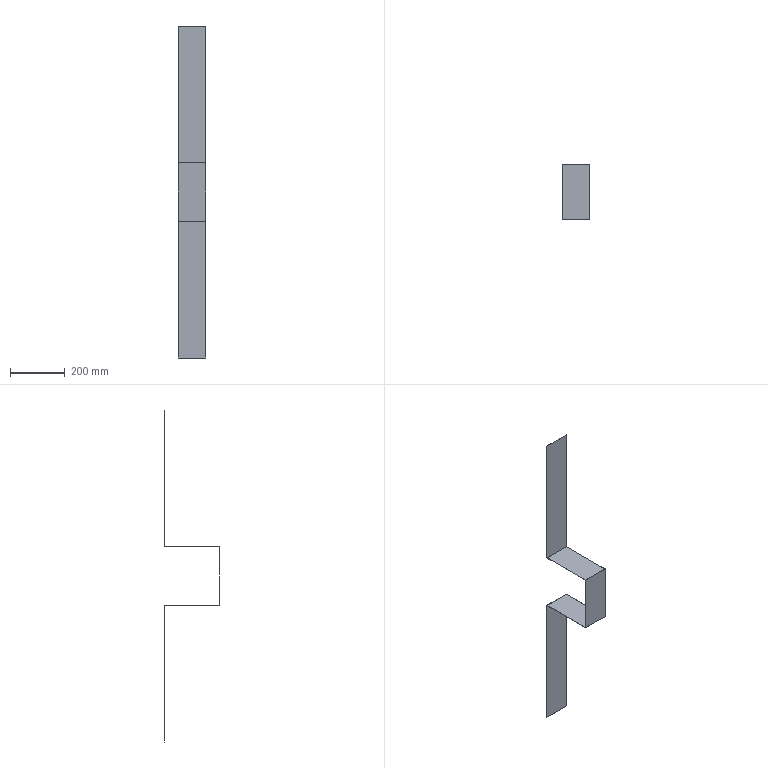Part | STEP file | 1 solid | 14 faces | box 100 x 200.5 x 1212 mm | volume 80600 mm3 | plane 14
STEP:
#1=CARTESIAN_POINT('',(0.,0.,0.));
#2=DIRECTION('',(0.,0.,1.));
#3=DIRECTION('',(1.,0.,0.));
#4=AXIS2_PLACEMENT_3D('',#1,#2,#3);
#5=CARTESIAN_POINT('',(-50.,0.25,0.));
#6=VERTEX_POINT('',#5);
#7=CARTESIAN_POINT('',(-50.,-0.25,0.));
#8=VERTEX_POINT('',#7);
#9=CARTESIAN_POINT('',(-50.,0.25,0.));
#10=DIRECTION('',(0.,-1.,0.));
#11=VECTOR('',#10,1.);
#12=LINE('',#9,#11);
#13=CARTESIAN_POINT('',(50.,0.25,0.));
#14=DIRECTION('',(0.,0.,-1.));
#15=DIRECTION('',(-1.,0.,0.));
#16=AXIS2_PLACEMENT_3D('',#13,#14,#15);
#17=PLANE('',#16);
#18=CARTESIAN_POINT('',(100.,0.));
#19=DIRECTION('',(0.,-1.));
#20=VECTOR('',#19,1.);
#21=LINE('',#18,#20);
#22=(GEOMETRIC_REPRESENTATION_CONTEXT(2)PARAMETRIC_REPRESENTATION_CONTEXT()REPRESENTATION_CONTEXT('',''));
#23=DEFINITIONAL_REPRESENTATION('',(#21),#22);
#24=PCURVE('',#17,#23);
#25=CARTESIAN_POINT('',(-50.,0.,0.));
#26=DIRECTION('',(1.,0.,0.));
#27=DIRECTION('',(0.,0.,-1.));
#28=AXIS2_PLACEMENT_3D('',#25,#26,#27);
#29=PLANE('',#28);
#30=CARTESIAN_POINT('',(0.,0.25));
#31=DIRECTION('',(0.,-1.));
#32=VECTOR('',#31,1.);
#33=LINE('',#30,#32);
#34=(GEOMETRIC_REPRESENTATION_CONTEXT(2)PARAMETRIC_REPRESENTATION_CONTEXT()REPRESENTATION_CONTEXT('',''));
#35=DEFINITIONAL_REPRESENTATION('',(#33),#34);
#36=PCURVE('',#29,#35);
#37=SURFACE_CURVE('',#12,(#24,#36),.PCURVE_S1.);
#38=EDGE_CURVE('',#6,#8,#37,.T.);
#39=ORIENTED_EDGE('',*,*,#38,.T.);
#40=CARTESIAN_POINT('',(50.,-0.25,0.));
#41=VERTEX_POINT('',#40);
#42=CARTESIAN_POINT('',(50.,-0.25,0.));
#43=DIRECTION('',(-1.,0.,0.));
#44=VECTOR('',#43,1.);
#45=LINE('',#42,#44);
#46=CARTESIAN_POINT('',(0.,-0.5));
#47=DIRECTION('',(1.,0.));
#48=VECTOR('',#47,1.);
#49=LINE('',#46,#48);
#50=(GEOMETRIC_REPRESENTATION_CONTEXT(2)PARAMETRIC_REPRESENTATION_CONTEXT()REPRESENTATION_CONTEXT('',''));
#51=DEFINITIONAL_REPRESENTATION('',(#49),#50);
#52=PCURVE('',#17,#51);
#53=CARTESIAN_POINT('',(50.,-0.25,0.));
#54=DIRECTION('',(0.,1.,0.));
#55=DIRECTION('',(0.,0.,1.));
#56=AXIS2_PLACEMENT_3D('',#53,#54,#55);
#57=PLANE('',#56);
#58=CARTESIAN_POINT('',(0.,0.));
#59=DIRECTION('',(0.,-1.));
#60=VECTOR('',#59,1.);
#61=LINE('',#58,#60);
#62=(GEOMETRIC_REPRESENTATION_CONTEXT(2)PARAMETRIC_REPRESENTATION_CONTEXT()REPRESENTATION_CONTEXT('',''));
#63=DEFINITIONAL_REPRESENTATION('',(#61),#62);
#64=PCURVE('',#57,#63);
#65=SURFACE_CURVE('',#45,(#52,#64),.PCURVE_S1.);
#66=EDGE_CURVE('',#41,#8,#65,.T.);
#67=ORIENTED_EDGE('',*,*,#66,.F.);
#68=CARTESIAN_POINT('',(50.,0.25,0.));
#69=VERTEX_POINT('',#68);
#70=CARTESIAN_POINT('',(50.,0.25,0.));
#71=DIRECTION('',(0.,-1.,0.));
#72=VECTOR('',#71,1.);
#73=LINE('',#70,#72);
#74=CARTESIAN_POINT('',(0.,0.));
#75=DIRECTION('',(0.,-1.));
#76=VECTOR('',#75,1.);
#77=LINE('',#74,#76);
#78=(GEOMETRIC_REPRESENTATION_CONTEXT(2)PARAMETRIC_REPRESENTATION_CONTEXT()REPRESENTATION_CONTEXT('',''));
#79=DEFINITIONAL_REPRESENTATION('',(#77),#78);
#80=PCURVE('',#17,#79);
#81=CARTESIAN_POINT('',(50.,0.,0.));
#82=DIRECTION('',(1.,0.,0.));
#83=DIRECTION('',(0.,0.,-1.));
#84=AXIS2_PLACEMENT_3D('',#81,#82,#83);
#85=PLANE('',#84);
#86=CARTESIAN_POINT('',(0.,0.25));
#87=DIRECTION('',(0.,-1.));
#88=VECTOR('',#87,1.);
#89=LINE('',#86,#88);
#90=(GEOMETRIC_REPRESENTATION_CONTEXT(2)PARAMETRIC_REPRESENTATION_CONTEXT()REPRESENTATION_CONTEXT('',''));
#91=DEFINITIONAL_REPRESENTATION('',(#89),#90);
#92=PCURVE('',#85,#91);
#93=SURFACE_CURVE('',#73,(#80,#92),.PCURVE_S1.);
#94=EDGE_CURVE('',#69,#41,#93,.T.);
#95=ORIENTED_EDGE('',*,*,#94,.F.);
#96=CARTESIAN_POINT('',(50.,0.25,0.));
#97=DIRECTION('',(-1.,0.,0.));
#98=VECTOR('',#97,1.);
#99=LINE('',#96,#98);
#100=CARTESIAN_POINT('',(0.,0.));
#101=DIRECTION('',(1.,0.));
#102=VECTOR('',#101,1.);
#103=LINE('',#100,#102);
#104=(GEOMETRIC_REPRESENTATION_CONTEXT(2)PARAMETRIC_REPRESENTATION_CONTEXT()REPRESENTATION_CONTEXT('',''));
#105=DEFINITIONAL_REPRESENTATION('',(#103),#104);
#106=PCURVE('',#17,#105);
#107=CARTESIAN_POINT('',(50.,0.25,0.));
#108=DIRECTION('',(0.,-1.,0.));
#109=DIRECTION('',(0.,0.,-1.));
#110=AXIS2_PLACEMENT_3D('',#107,#108,#109);
#111=PLANE('',#110);
#112=CARTESIAN_POINT('',(0.,0.));
#113=DIRECTION('',(0.,-1.));
#114=VECTOR('',#113,1.);
#115=LINE('',#112,#114);
#116=(GEOMETRIC_REPRESENTATION_CONTEXT(2)PARAMETRIC_REPRESENTATION_CONTEXT()REPRESENTATION_CONTEXT('',''));
#117=DEFINITIONAL_REPRESENTATION('',(#115),#116);
#118=PCURVE('',#111,#117);
#119=SURFACE_CURVE('',#99,(#106,#118),.PCURVE_S1.);
#120=EDGE_CURVE('',#69,#6,#119,.T.);
#121=ORIENTED_EDGE('',*,*,#120,.T.);
#122=EDGE_LOOP('',(#39,#67,#95,#121));
#123=FACE_BOUND('',#122,.T.);
#124=ADVANCED_FACE('',(#123),#17,.F.);
#125=CARTESIAN_POINT('',(-50.,-0.25,-499.5));
#126=VERTEX_POINT('',#125);
#127=CARTESIAN_POINT('',(-50.,-0.25,0.));
#128=DIRECTION('',(0.,0.,-1.));
#129=VECTOR('',#128,1.);
#130=LINE('',#127,#129);
#131=CARTESIAN_POINT('',(0.,-100.));
#132=DIRECTION('',(-1.,0.));
#133=VECTOR('',#132,1.);
#134=LINE('',#131,#133);
#135=(GEOMETRIC_REPRESENTATION_CONTEXT(2)PARAMETRIC_REPRESENTATION_CONTEXT()REPRESENTATION_CONTEXT('',''));
#136=DEFINITIONAL_REPRESENTATION('',(#134),#135);
#137=PCURVE('',#57,#136);
#138=CARTESIAN_POINT('',(0.,-0.25));
#139=DIRECTION('',(1.,0.));
#140=VECTOR('',#139,1.);
#141=LINE('',#138,#140);
#142=(GEOMETRIC_REPRESENTATION_CONTEXT(2)PARAMETRIC_REPRESENTATION_CONTEXT()REPRESENTATION_CONTEXT('',''));
#143=DEFINITIONAL_REPRESENTATION('',(#141),#142);
#144=PCURVE('',#29,#143);
#145=SURFACE_CURVE('',#130,(#137,#144),.PCURVE_S1.);
#146=EDGE_CURVE('',#8,#126,#145,.T.);
#147=ORIENTED_EDGE('',*,*,#146,.T.);
#148=CARTESIAN_POINT('',(50.,-0.25,-499.5));
#149=VERTEX_POINT('',#148);
#150=CARTESIAN_POINT('',(50.,-0.25,-499.5));
#151=DIRECTION('',(-1.,0.,0.));
#152=VECTOR('',#151,1.);
#153=LINE('',#150,#152);
#154=CARTESIAN_POINT('',(-499.5,0.));
#155=DIRECTION('',(0.,-1.));
#156=VECTOR('',#155,1.);
#157=LINE('',#154,#156);
#158=(GEOMETRIC_REPRESENTATION_CONTEXT(2)PARAMETRIC_REPRESENTATION_CONTEXT()REPRESENTATION_CONTEXT('',''));
#159=DEFINITIONAL_REPRESENTATION('',(#157),#158);
#160=PCURVE('',#57,#159);
#161=CARTESIAN_POINT('',(50.,-0.25,-499.5));
#162=DIRECTION('',(0.,0.,-1.));
#163=DIRECTION('',(-1.,0.,0.));
#164=AXIS2_PLACEMENT_3D('',#161,#162,#163);
#165=PLANE('',#164);
#166=CARTESIAN_POINT('',(0.,0.));
#167=DIRECTION('',(1.,0.));
#168=VECTOR('',#167,1.);
#169=LINE('',#166,#168);
#170=(GEOMETRIC_REPRESENTATION_CONTEXT(2)PARAMETRIC_REPRESENTATION_CONTEXT()REPRESENTATION_CONTEXT('',''));
#171=DEFINITIONAL_REPRESENTATION('',(#169),#170);
#172=PCURVE('',#165,#171);
#173=SURFACE_CURVE('',#153,(#160,#172),.PCURVE_S1.);
#174=EDGE_CURVE('',#149,#126,#173,.T.);
#175=ORIENTED_EDGE('',*,*,#174,.F.);
#176=CARTESIAN_POINT('',(50.,-0.25,0.));
#177=DIRECTION('',(0.,0.,-1.));
#178=VECTOR('',#177,1.);
#179=LINE('',#176,#178);
#180=CARTESIAN_POINT('',(0.,0.));
#181=DIRECTION('',(-1.,0.));
#182=VECTOR('',#181,1.);
#183=LINE('',#180,#182);
#184=(GEOMETRIC_REPRESENTATION_CONTEXT(2)PARAMETRIC_REPRESENTATION_CONTEXT()REPRESENTATION_CONTEXT('',''));
#185=DEFINITIONAL_REPRESENTATION('',(#183),#184);
#186=PCURVE('',#57,#185);
#187=CARTESIAN_POINT('',(0.,-0.25));
#188=DIRECTION('',(1.,0.));
#189=VECTOR('',#188,1.);
#190=LINE('',#187,#189);
#191=(GEOMETRIC_REPRESENTATION_CONTEXT(2)PARAMETRIC_REPRESENTATION_CONTEXT()REPRESENTATION_CONTEXT('',''));
#192=DEFINITIONAL_REPRESENTATION('',(#190),#191);
#193=PCURVE('',#85,#192);
#194=SURFACE_CURVE('',#179,(#186,#193),.PCURVE_S1.);
#195=EDGE_CURVE('',#41,#149,#194,.T.);
#196=ORIENTED_EDGE('',*,*,#195,.F.);
#197=ORIENTED_EDGE('',*,*,#66,.T.);
#198=EDGE_LOOP('',(#147,#175,#196,#197));
#199=FACE_BOUND('',#198,.T.);
#200=ADVANCED_FACE('',(#199),#57,.F.);
#201=CARTESIAN_POINT('',(-50.,-200.25,-499.5));
#202=VERTEX_POINT('',#201);
#203=CARTESIAN_POINT('',(-50.,-0.25,-499.5));
#204=DIRECTION('',(0.,-1.,0.));
#205=VECTOR('',#204,1.);
#206=LINE('',#203,#205);
#207=CARTESIAN_POINT('',(100.,0.));
#208=DIRECTION('',(0.,-1.));
#209=VECTOR('',#208,1.);
#210=LINE('',#207,#209);
#211=(GEOMETRIC_REPRESENTATION_CONTEXT(2)PARAMETRIC_REPRESENTATION_CONTEXT()REPRESENTATION_CONTEXT('',''));
#212=DEFINITIONAL_REPRESENTATION('',(#210),#211);
#213=PCURVE('',#165,#212);
#214=CARTESIAN_POINT('',(499.5,-0.25));
#215=DIRECTION('',(0.,-1.));
#216=VECTOR('',#215,1.);
#217=LINE('',#214,#216);
#218=(GEOMETRIC_REPRESENTATION_CONTEXT(2)PARAMETRIC_REPRESENTATION_CONTEXT()REPRESENTATION_CONTEXT('',''));
#219=DEFINITIONAL_REPRESENTATION('',(#217),#218);
#220=PCURVE('',#29,#219);
#221=SURFACE_CURVE('',#206,(#213,#220),.PCURVE_S1.);
#222=EDGE_CURVE('',#126,#202,#221,.T.);
#223=ORIENTED_EDGE('',*,*,#222,.T.);
#224=CARTESIAN_POINT('',(50.,-200.25,-499.5));
#225=VERTEX_POINT('',#224);
#226=CARTESIAN_POINT('',(50.,-200.25,-499.5));
#227=DIRECTION('',(-1.,0.,0.));
#228=VECTOR('',#227,1.);
#229=LINE('',#226,#228);
#230=CARTESIAN_POINT('',(0.,-200.));
#231=DIRECTION('',(1.,0.));
#232=VECTOR('',#231,1.);
#233=LINE('',#230,#232);
#234=(GEOMETRIC_REPRESENTATION_CONTEXT(2)PARAMETRIC_REPRESENTATION_CONTEXT()REPRESENTATION_CONTEXT('',''));
#235=DEFINITIONAL_REPRESENTATION('',(#233),#234);
#236=PCURVE('',#165,#235);
#237=CARTESIAN_POINT('',(50.,-200.25,-499.5));
#238=DIRECTION('',(0.,1.,0.));
#239=DIRECTION('',(0.,0.,1.));
#240=AXIS2_PLACEMENT_3D('',#237,#238,#239);
#241=PLANE('',#240);
#242=CARTESIAN_POINT('',(0.,0.));
#243=DIRECTION('',(0.,-1.));
#244=VECTOR('',#243,1.);
#245=LINE('',#242,#244);
#246=(GEOMETRIC_REPRESENTATION_CONTEXT(2)PARAMETRIC_REPRESENTATION_CONTEXT()REPRESENTATION_CONTEXT('',''));
#247=DEFINITIONAL_REPRESENTATION('',(#245),#246);
#248=PCURVE('',#241,#247);
#249=SURFACE_CURVE('',#229,(#236,#248),.PCURVE_S1.);
#250=EDGE_CURVE('',#225,#202,#249,.T.);
#251=ORIENTED_EDGE('',*,*,#250,.F.);
#252=CARTESIAN_POINT('',(50.,-0.25,-499.5));
#253=DIRECTION('',(0.,-1.,0.));
#254=VECTOR('',#253,1.);
#255=LINE('',#252,#254);
#256=CARTESIAN_POINT('',(0.,0.));
#257=DIRECTION('',(0.,-1.));
#258=VECTOR('',#257,1.);
#259=LINE('',#256,#258);
#260=(GEOMETRIC_REPRESENTATION_CONTEXT(2)PARAMETRIC_REPRESENTATION_CONTEXT()REPRESENTATION_CONTEXT('',''));
#261=DEFINITIONAL_REPRESENTATION('',(#259),#260);
#262=PCURVE('',#165,#261);
#263=CARTESIAN_POINT('',(499.5,-0.25));
#264=DIRECTION('',(0.,-1.));
#265=VECTOR('',#264,1.);
#266=LINE('',#263,#265);
#267=(GEOMETRIC_REPRESENTATION_CONTEXT(2)PARAMETRIC_REPRESENTATION_CONTEXT()REPRESENTATION_CONTEXT('',''));
#268=DEFINITIONAL_REPRESENTATION('',(#266),#267);
#269=PCURVE('',#85,#268);
#270=SURFACE_CURVE('',#255,(#262,#269),.PCURVE_S1.);
#271=EDGE_CURVE('',#149,#225,#270,.T.);
#272=ORIENTED_EDGE('',*,*,#271,.F.);
#273=ORIENTED_EDGE('',*,*,#174,.T.);
#274=EDGE_LOOP('',(#223,#251,#272,#273));
#275=FACE_BOUND('',#274,.T.);
#276=ADVANCED_FACE('',(#275),#165,.F.);
#277=CARTESIAN_POINT('',(-50.,-200.25,-712.5));
#278=VERTEX_POINT('',#277);
#279=CARTESIAN_POINT('',(-50.,-200.25,-499.5));
#280=DIRECTION('',(0.,0.,-1.));
#281=VECTOR('',#280,1.);
#282=LINE('',#279,#281);
#283=CARTESIAN_POINT('',(0.,-100.));
#284=DIRECTION('',(-1.,0.));
#285=VECTOR('',#284,1.);
#286=LINE('',#283,#285);
#287=(GEOMETRIC_REPRESENTATION_CONTEXT(2)PARAMETRIC_REPRESENTATION_CONTEXT()REPRESENTATION_CONTEXT('',''));
#288=DEFINITIONAL_REPRESENTATION('',(#286),#287);
#289=PCURVE('',#241,#288);
#290=CARTESIAN_POINT('',(499.5,-200.25));
#291=DIRECTION('',(1.,0.));
#292=VECTOR('',#291,1.);
#293=LINE('',#290,#292);
#294=(GEOMETRIC_REPRESENTATION_CONTEXT(2)PARAMETRIC_REPRESENTATION_CONTEXT()REPRESENTATION_CONTEXT('',''));
#295=DEFINITIONAL_REPRESENTATION('',(#293),#294);
#296=PCURVE('',#29,#295);
#297=SURFACE_CURVE('',#282,(#289,#296),.PCURVE_S1.);
#298=EDGE_CURVE('',#202,#278,#297,.T.);
#299=ORIENTED_EDGE('',*,*,#298,.T.);
#300=CARTESIAN_POINT('',(50.,-200.25,-712.5));
#301=VERTEX_POINT('',#300);
#302=CARTESIAN_POINT('',(50.,-200.25,-712.5));
#303=DIRECTION('',(-1.,0.,0.));
#304=VECTOR('',#303,1.);
#305=LINE('',#302,#304);
#306=CARTESIAN_POINT('',(-213.,0.));
#307=DIRECTION('',(0.,-1.));
#308=VECTOR('',#307,1.);
#309=LINE('',#306,#308);
#310=(GEOMETRIC_REPRESENTATION_CONTEXT(2)PARAMETRIC_REPRESENTATION_CONTEXT()REPRESENTATION_CONTEXT('',''));
#311=DEFINITIONAL_REPRESENTATION('',(#309),#310);
#312=PCURVE('',#241,#311);
#313=CARTESIAN_POINT('',(50.,-200.25,-712.5));
#314=DIRECTION('',(0.,0.,1.));
#315=DIRECTION('',(1.,0.,0.));
#316=AXIS2_PLACEMENT_3D('',#313,#314,#315);
#317=PLANE('',#316);
#318=CARTESIAN_POINT('',(0.,0.));
#319=DIRECTION('',(-1.,0.));
#320=VECTOR('',#319,1.);
#321=LINE('',#318,#320);
#322=(GEOMETRIC_REPRESENTATION_CONTEXT(2)PARAMETRIC_REPRESENTATION_CONTEXT()REPRESENTATION_CONTEXT('',''));
#323=DEFINITIONAL_REPRESENTATION('',(#321),#322);
#324=PCURVE('',#317,#323);
#325=SURFACE_CURVE('',#305,(#312,#324),.PCURVE_S1.);
#326=EDGE_CURVE('',#301,#278,#325,.T.);
#327=ORIENTED_EDGE('',*,*,#326,.F.);
#328=CARTESIAN_POINT('',(50.,-200.25,-499.5));
#329=DIRECTION('',(0.,0.,-1.));
#330=VECTOR('',#329,1.);
#331=LINE('',#328,#330);
#332=CARTESIAN_POINT('',(0.,0.));
#333=DIRECTION('',(-1.,0.));
#334=VECTOR('',#333,1.);
#335=LINE('',#332,#334);
#336=(GEOMETRIC_REPRESENTATION_CONTEXT(2)PARAMETRIC_REPRESENTATION_CONTEXT()REPRESENTATION_CONTEXT('',''));
#337=DEFINITIONAL_REPRESENTATION('',(#335),#336);
#338=PCURVE('',#241,#337);
#339=CARTESIAN_POINT('',(499.5,-200.25));
#340=DIRECTION('',(1.,0.));
#341=VECTOR('',#340,1.);
#342=LINE('',#339,#341);
#343=(GEOMETRIC_REPRESENTATION_CONTEXT(2)PARAMETRIC_REPRESENTATION_CONTEXT()REPRESENTATION_CONTEXT('',''));
#344=DEFINITIONAL_REPRESENTATION('',(#342),#343);
#345=PCURVE('',#85,#344);
#346=SURFACE_CURVE('',#331,(#338,#345),.PCURVE_S1.);
#347=EDGE_CURVE('',#225,#301,#346,.T.);
#348=ORIENTED_EDGE('',*,*,#347,.F.);
#349=ORIENTED_EDGE('',*,*,#250,.T.);
#350=EDGE_LOOP('',(#299,#327,#348,#349));
#351=FACE_BOUND('',#350,.T.);
#352=ADVANCED_FACE('',(#351),#241,.F.);
#353=CARTESIAN_POINT('',(-50.,-0.25,-712.5));
#354=VERTEX_POINT('',#353);
#355=CARTESIAN_POINT('',(-50.,-200.25,-712.5));
#356=DIRECTION('',(0.,1.,0.));
#357=VECTOR('',#356,1.);
#358=LINE('',#355,#357);
#359=CARTESIAN_POINT('',(-100.,0.));
#360=DIRECTION('',(0.,1.));
#361=VECTOR('',#360,1.);
#362=LINE('',#359,#361);
#363=(GEOMETRIC_REPRESENTATION_CONTEXT(2)PARAMETRIC_REPRESENTATION_CONTEXT()REPRESENTATION_CONTEXT('',''));
#364=DEFINITIONAL_REPRESENTATION('',(#362),#363);
#365=PCURVE('',#317,#364);
#366=CARTESIAN_POINT('',(712.5,-200.25));
#367=DIRECTION('',(0.,1.));
#368=VECTOR('',#367,1.);
#369=LINE('',#366,#368);
#370=(GEOMETRIC_REPRESENTATION_CONTEXT(2)PARAMETRIC_REPRESENTATION_CONTEXT()REPRESENTATION_CONTEXT('',''));
#371=DEFINITIONAL_REPRESENTATION('',(#369),#370);
#372=PCURVE('',#29,#371);
#373=SURFACE_CURVE('',#358,(#365,#372),.PCURVE_S1.);
#374=EDGE_CURVE('',#278,#354,#373,.T.);
#375=ORIENTED_EDGE('',*,*,#374,.T.);
#376=CARTESIAN_POINT('',(50.,-0.25,-712.5));
#377=VERTEX_POINT('',#376);
#378=CARTESIAN_POINT('',(50.,-0.25,-712.5));
#379=DIRECTION('',(-1.,0.,0.));
#380=VECTOR('',#379,1.);
#381=LINE('',#378,#380);
#382=CARTESIAN_POINT('',(0.,200.));
#383=DIRECTION('',(-1.,0.));
#384=VECTOR('',#383,1.);
#385=LINE('',#382,#384);
#386=(GEOMETRIC_REPRESENTATION_CONTEXT(2)PARAMETRIC_REPRESENTATION_CONTEXT()REPRESENTATION_CONTEXT('',''));
#387=DEFINITIONAL_REPRESENTATION('',(#385),#386);
#388=PCURVE('',#317,#387);
#389=CARTESIAN_POINT('',(50.,-0.25,-712.5));
#390=DIRECTION('',(0.,1.,0.));
#391=DIRECTION('',(0.,0.,1.));
#392=AXIS2_PLACEMENT_3D('',#389,#390,#391);
#393=PLANE('',#392);
#394=CARTESIAN_POINT('',(0.,0.));
#395=DIRECTION('',(0.,-1.));
#396=VECTOR('',#395,1.);
#397=LINE('',#394,#396);
#398=(GEOMETRIC_REPRESENTATION_CONTEXT(2)PARAMETRIC_REPRESENTATION_CONTEXT()REPRESENTATION_CONTEXT('',''));
#399=DEFINITIONAL_REPRESENTATION('',(#397),#398);
#400=PCURVE('',#393,#399);
#401=SURFACE_CURVE('',#381,(#388,#400),.PCURVE_S1.);
#402=EDGE_CURVE('',#377,#354,#401,.T.);
#403=ORIENTED_EDGE('',*,*,#402,.F.);
#404=CARTESIAN_POINT('',(50.,-200.25,-712.5));
#405=DIRECTION('',(0.,1.,0.));
#406=VECTOR('',#405,1.);
#407=LINE('',#404,#406);
#408=CARTESIAN_POINT('',(0.,0.));
#409=DIRECTION('',(0.,1.));
#410=VECTOR('',#409,1.);
#411=LINE('',#408,#410);
#412=(GEOMETRIC_REPRESENTATION_CONTEXT(2)PARAMETRIC_REPRESENTATION_CONTEXT()REPRESENTATION_CONTEXT('',''));
#413=DEFINITIONAL_REPRESENTATION('',(#411),#412);
#414=PCURVE('',#317,#413);
#415=CARTESIAN_POINT('',(712.5,-200.25));
#416=DIRECTION('',(0.,1.));
#417=VECTOR('',#416,1.);
#418=LINE('',#415,#417);
#419=(GEOMETRIC_REPRESENTATION_CONTEXT(2)PARAMETRIC_REPRESENTATION_CONTEXT()REPRESENTATION_CONTEXT('',''));
#420=DEFINITIONAL_REPRESENTATION('',(#418),#419);
#421=PCURVE('',#85,#420);
#422=SURFACE_CURVE('',#407,(#414,#421),.PCURVE_S1.);
#423=EDGE_CURVE('',#301,#377,#422,.T.);
#424=ORIENTED_EDGE('',*,*,#423,.F.);
#425=ORIENTED_EDGE('',*,*,#326,.T.);
#426=EDGE_LOOP('',(#375,#403,#424,#425));
#427=FACE_BOUND('',#426,.T.);
#428=ADVANCED_FACE('',(#427),#317,.F.);
#429=CARTESIAN_POINT('',(-50.,-0.25,-1212.));
#430=VERTEX_POINT('',#429);
#431=CARTESIAN_POINT('',(-50.,-0.25,-712.5));
#432=DIRECTION('',(0.,0.,-1.));
#433=VECTOR('',#432,1.);
#434=LINE('',#431,#433);
#435=CARTESIAN_POINT('',(0.,-100.));
#436=DIRECTION('',(-1.,0.));
#437=VECTOR('',#436,1.);
#438=LINE('',#435,#437);
#439=(GEOMETRIC_REPRESENTATION_CONTEXT(2)PARAMETRIC_REPRESENTATION_CONTEXT()REPRESENTATION_CONTEXT('',''));
#440=DEFINITIONAL_REPRESENTATION('',(#438),#439);
#441=PCURVE('',#393,#440);
#442=CARTESIAN_POINT('',(712.5,-0.25));
#443=DIRECTION('',(1.,0.));
#444=VECTOR('',#443,1.);
#445=LINE('',#442,#444);
#446=(GEOMETRIC_REPRESENTATION_CONTEXT(2)PARAMETRIC_REPRESENTATION_CONTEXT()REPRESENTATION_CONTEXT('',''));
#447=DEFINITIONAL_REPRESENTATION('',(#445),#446);
#448=PCURVE('',#29,#447);
#449=SURFACE_CURVE('',#434,(#441,#448),.PCURVE_S1.);
#450=EDGE_CURVE('',#354,#430,#449,.T.);
#451=ORIENTED_EDGE('',*,*,#450,.T.);
#452=CARTESIAN_POINT('',(50.,-0.25,-1212.));
#453=VERTEX_POINT('',#452);
#454=CARTESIAN_POINT('',(50.,-0.25,-1212.));
#455=DIRECTION('',(-1.,0.,0.));
#456=VECTOR('',#455,1.);
#457=LINE('',#454,#456);
#458=CARTESIAN_POINT('',(-499.5,0.));
#459=DIRECTION('',(0.,-1.));
#460=VECTOR('',#459,1.);
#461=LINE('',#458,#460);
#462=(GEOMETRIC_REPRESENTATION_CONTEXT(2)PARAMETRIC_REPRESENTATION_CONTEXT()REPRESENTATION_CONTEXT('',''));
#463=DEFINITIONAL_REPRESENTATION('',(#461),#462);
#464=PCURVE('',#393,#463);
#465=CARTESIAN_POINT('',(50.,0.25,-1212.));
#466=DIRECTION('',(0.,0.,1.));
#467=DIRECTION('',(1.,0.,0.));
#468=AXIS2_PLACEMENT_3D('',#465,#466,#467);
#469=PLANE('',#468);
#470=CARTESIAN_POINT('',(0.,-0.5));
#471=DIRECTION('',(-1.,0.));
#472=VECTOR('',#471,1.);
#473=LINE('',#470,#472);
#474=(GEOMETRIC_REPRESENTATION_CONTEXT(2)PARAMETRIC_REPRESENTATION_CONTEXT()REPRESENTATION_CONTEXT('',''));
#475=DEFINITIONAL_REPRESENTATION('',(#473),#474);
#476=PCURVE('',#469,#475);
#477=SURFACE_CURVE('',#457,(#464,#476),.PCURVE_S1.);
#478=EDGE_CURVE('',#453,#430,#477,.T.);
#479=ORIENTED_EDGE('',*,*,#478,.F.);
#480=CARTESIAN_POINT('',(50.,-0.25,-712.5));
#481=DIRECTION('',(0.,0.,-1.));
#482=VECTOR('',#481,1.);
#483=LINE('',#480,#482);
#484=CARTESIAN_POINT('',(0.,0.));
#485=DIRECTION('',(-1.,0.));
#486=VECTOR('',#485,1.);
#487=LINE('',#484,#486);
#488=(GEOMETRIC_REPRESENTATION_CONTEXT(2)PARAMETRIC_REPRESENTATION_CONTEXT()REPRESENTATION_CONTEXT('',''));
#489=DEFINITIONAL_REPRESENTATION('',(#487),#488);
#490=PCURVE('',#393,#489);
#491=CARTESIAN_POINT('',(712.5,-0.25));
#492=DIRECTION('',(1.,0.));
#493=VECTOR('',#492,1.);
#494=LINE('',#491,#493);
#495=(GEOMETRIC_REPRESENTATION_CONTEXT(2)PARAMETRIC_REPRESENTATION_CONTEXT()REPRESENTATION_CONTEXT('',''));
#496=DEFINITIONAL_REPRESENTATION('',(#494),#495);
#497=PCURVE('',#85,#496);
#498=SURFACE_CURVE('',#483,(#490,#497),.PCURVE_S1.);
#499=EDGE_CURVE('',#377,#453,#498,.T.);
#500=ORIENTED_EDGE('',*,*,#499,.F.);
#501=ORIENTED_EDGE('',*,*,#402,.T.);
#502=EDGE_LOOP('',(#451,#479,#500,#501));
#503=FACE_BOUND('',#502,.T.);
#504=ADVANCED_FACE('',(#503),#393,.F.);
#505=CARTESIAN_POINT('',(-50.,0.25,-1212.));
#506=VERTEX_POINT('',#505);
#507=CARTESIAN_POINT('',(-50.,0.25,-1212.));
#508=DIRECTION('',(0.,1.,0.));
#509=VECTOR('',#508,1.);
#510=LINE('',#507,#509);
#511=CARTESIAN_POINT('',(-100.,0.));
#512=DIRECTION('',(0.,1.));
#513=VECTOR('',#512,1.);
#514=LINE('',#511,#513);
#515=(GEOMETRIC_REPRESENTATION_CONTEXT(2)PARAMETRIC_REPRESENTATION_CONTEXT()REPRESENTATION_CONTEXT('',''));
#516=DEFINITIONAL_REPRESENTATION('',(#514),#515);
#517=PCURVE('',#469,#516);
#518=CARTESIAN_POINT('',(1212.,0.25));
#519=DIRECTION('',(0.,1.));
#520=VECTOR('',#519,1.);
#521=LINE('',#518,#520);
#522=(GEOMETRIC_REPRESENTATION_CONTEXT(2)PARAMETRIC_REPRESENTATION_CONTEXT()REPRESENTATION_CONTEXT('',''));
#523=DEFINITIONAL_REPRESENTATION('',(#521),#522);
#524=PCURVE('',#29,#523);
#525=SURFACE_CURVE('',#510,(#517,#524),.PCURVE_S1.);
#526=EDGE_CURVE('',#430,#506,#525,.T.);
#527=ORIENTED_EDGE('',*,*,#526,.T.);
#528=CARTESIAN_POINT('',(50.,0.25,-1212.));
#529=VERTEX_POINT('',#528);
#530=CARTESIAN_POINT('',(50.,0.25,-1212.));
#531=DIRECTION('',(-1.,0.,0.));
#532=VECTOR('',#531,1.);
#533=LINE('',#530,#532);
#534=CARTESIAN_POINT('',(0.,0.));
#535=DIRECTION('',(-1.,0.));
#536=VECTOR('',#535,1.);
#537=LINE('',#534,#536);
#538=(GEOMETRIC_REPRESENTATION_CONTEXT(2)PARAMETRIC_REPRESENTATION_CONTEXT()REPRESENTATION_CONTEXT('',''));
#539=DEFINITIONAL_REPRESENTATION('',(#537),#538);
#540=PCURVE('',#469,#539);
#541=CARTESIAN_POINT('',(50.,0.25,-712.));
#542=DIRECTION('',(0.,-1.,0.));
#543=DIRECTION('',(0.,0.,-1.));
#544=AXIS2_PLACEMENT_3D('',#541,#542,#543);
#545=PLANE('',#544);
#546=CARTESIAN_POINT('',(500.,0.));
#547=DIRECTION('',(0.,-1.));
#548=VECTOR('',#547,1.);
#549=LINE('',#546,#548);
#550=(GEOMETRIC_REPRESENTATION_CONTEXT(2)PARAMETRIC_REPRESENTATION_CONTEXT()REPRESENTATION_CONTEXT('',''));
#551=DEFINITIONAL_REPRESENTATION('',(#549),#550);
#552=PCURVE('',#545,#551);
#553=SURFACE_CURVE('',#533,(#540,#552),.PCURVE_S1.);
#554=EDGE_CURVE('',#529,#506,#553,.T.);
#555=ORIENTED_EDGE('',*,*,#554,.F.);
#556=CARTESIAN_POINT('',(50.,0.25,-1212.));
#557=DIRECTION('',(0.,1.,0.));
#558=VECTOR('',#557,1.);
#559=LINE('',#556,#558);
#560=CARTESIAN_POINT('',(0.,0.));
#561=DIRECTION('',(0.,1.));
#562=VECTOR('',#561,1.);
#563=LINE('',#560,#562);
#564=(GEOMETRIC_REPRESENTATION_CONTEXT(2)PARAMETRIC_REPRESENTATION_CONTEXT()REPRESENTATION_CONTEXT('',''));
#565=DEFINITIONAL_REPRESENTATION('',(#563),#564);
#566=PCURVE('',#469,#565);
#567=CARTESIAN_POINT('',(1212.,0.25));
#568=DIRECTION('',(0.,1.));
#569=VECTOR('',#568,1.);
#570=LINE('',#567,#569);
#571=(GEOMETRIC_REPRESENTATION_CONTEXT(2)PARAMETRIC_REPRESENTATION_CONTEXT()REPRESENTATION_CONTEXT('',''));
#572=DEFINITIONAL_REPRESENTATION('',(#570),#571);
#573=PCURVE('',#85,#572);
#574=SURFACE_CURVE('',#559,(#566,#573),.PCURVE_S1.);
#575=EDGE_CURVE('',#453,#529,#574,.T.);
#576=ORIENTED_EDGE('',*,*,#575,.F.);
#577=ORIENTED_EDGE('',*,*,#478,.T.);
#578=EDGE_LOOP('',(#527,#555,#576,#577));
#579=FACE_BOUND('',#578,.T.);
#580=ADVANCED_FACE('',(#579),#469,.F.);
#581=CARTESIAN_POINT('',(-50.,0.25,-712.));
#582=VERTEX_POINT('',#581);
#583=CARTESIAN_POINT('',(-50.,0.25,-712.));
#584=DIRECTION('',(0.,0.,1.));
#585=VECTOR('',#584,1.);
#586=LINE('',#583,#585);
#587=CARTESIAN_POINT('',(0.,-100.));
#588=DIRECTION('',(-1.,0.));
#589=VECTOR('',#588,1.);
#590=LINE('',#587,#589);
#591=(GEOMETRIC_REPRESENTATION_CONTEXT(2)PARAMETRIC_REPRESENTATION_CONTEXT()REPRESENTATION_CONTEXT('',''));
#592=DEFINITIONAL_REPRESENTATION('',(#590),#591);
#593=PCURVE('',#545,#592);
#594=CARTESIAN_POINT('',(712.,0.25));
#595=DIRECTION('',(-1.,0.));
#596=VECTOR('',#595,1.);
#597=LINE('',#594,#596);
#598=(GEOMETRIC_REPRESENTATION_CONTEXT(2)PARAMETRIC_REPRESENTATION_CONTEXT()REPRESENTATION_CONTEXT('',''));
#599=DEFINITIONAL_REPRESENTATION('',(#597),#598);
#600=PCURVE('',#29,#599);
#601=SURFACE_CURVE('',#586,(#593,#600),.PCURVE_S1.);
#602=EDGE_CURVE('',#506,#582,#601,.T.);
#603=ORIENTED_EDGE('',*,*,#602,.T.);
#604=CARTESIAN_POINT('',(50.,0.25,-712.));
#605=VERTEX_POINT('',#604);
#606=CARTESIAN_POINT('',(50.,0.25,-712.));
#607=DIRECTION('',(-1.,0.,0.));
#608=VECTOR('',#607,1.);
#609=LINE('',#606,#608);
#610=CARTESIAN_POINT('',(0.,0.));
#611=DIRECTION('',(0.,-1.));
#612=VECTOR('',#611,1.);
#613=LINE('',#610,#612);
#614=(GEOMETRIC_REPRESENTATION_CONTEXT(2)PARAMETRIC_REPRESENTATION_CONTEXT()REPRESENTATION_CONTEXT('',''));
#615=DEFINITIONAL_REPRESENTATION('',(#613),#614);
#616=PCURVE('',#545,#615);
#617=CARTESIAN_POINT('',(50.,-199.75,-712.));
#618=DIRECTION('',(0.,0.,-1.));
#619=DIRECTION('',(-1.,0.,0.));
#620=AXIS2_PLACEMENT_3D('',#617,#618,#619);
#621=PLANE('',#620);
#622=CARTESIAN_POINT('',(0.,200.));
#623=DIRECTION('',(1.,0.));
#624=VECTOR('',#623,1.);
#625=LINE('',#622,#624);
#626=(GEOMETRIC_REPRESENTATION_CONTEXT(2)PARAMETRIC_REPRESENTATION_CONTEXT()REPRESENTATION_CONTEXT('',''));
#627=DEFINITIONAL_REPRESENTATION('',(#625),#626);
#628=PCURVE('',#621,#627);
#629=SURFACE_CURVE('',#609,(#616,#628),.PCURVE_S1.);
#630=EDGE_CURVE('',#605,#582,#629,.T.);
#631=ORIENTED_EDGE('',*,*,#630,.F.);
#632=CARTESIAN_POINT('',(50.,0.25,-712.));
#633=DIRECTION('',(0.,0.,1.));
#634=VECTOR('',#633,1.);
#635=LINE('',#632,#634);
#636=CARTESIAN_POINT('',(0.,0.));
#637=DIRECTION('',(-1.,0.));
#638=VECTOR('',#637,1.);
#639=LINE('',#636,#638);
#640=(GEOMETRIC_REPRESENTATION_CONTEXT(2)PARAMETRIC_REPRESENTATION_CONTEXT()REPRESENTATION_CONTEXT('',''));
#641=DEFINITIONAL_REPRESENTATION('',(#639),#640);
#642=PCURVE('',#545,#641);
#643=CARTESIAN_POINT('',(712.,0.25));
#644=DIRECTION('',(-1.,0.));
#645=VECTOR('',#644,1.);
#646=LINE('',#643,#645);
#647=(GEOMETRIC_REPRESENTATION_CONTEXT(2)PARAMETRIC_REPRESENTATION_CONTEXT()REPRESENTATION_CONTEXT('',''));
#648=DEFINITIONAL_REPRESENTATION('',(#646),#647);
#649=PCURVE('',#85,#648);
#650=SURFACE_CURVE('',#635,(#642,#649),.PCURVE_S1.);
#651=EDGE_CURVE('',#529,#605,#650,.T.);
#652=ORIENTED_EDGE('',*,*,#651,.F.);
#653=ORIENTED_EDGE('',*,*,#554,.T.);
#654=EDGE_LOOP('',(#603,#631,#652,#653));
#655=FACE_BOUND('',#654,.T.);
#656=ADVANCED_FACE('',(#655),#545,.F.);
#657=CARTESIAN_POINT('',(-50.,-199.75,-712.));
#658=VERTEX_POINT('',#657);
#659=CARTESIAN_POINT('',(-50.,-199.75,-712.));
#660=DIRECTION('',(0.,-1.,0.));
#661=VECTOR('',#660,1.);
#662=LINE('',#659,#661);
#663=CARTESIAN_POINT('',(100.,0.));
#664=DIRECTION('',(0.,-1.));
#665=VECTOR('',#664,1.);
#666=LINE('',#663,#665);
#667=(GEOMETRIC_REPRESENTATION_CONTEXT(2)PARAMETRIC_REPRESENTATION_CONTEXT()REPRESENTATION_CONTEXT('',''));
#668=DEFINITIONAL_REPRESENTATION('',(#666),#667);
#669=PCURVE('',#621,#668);
#670=CARTESIAN_POINT('',(712.,-199.75));
#671=DIRECTION('',(0.,-1.));
#672=VECTOR('',#671,1.);
#673=LINE('',#670,#672);
#674=(GEOMETRIC_REPRESENTATION_CONTEXT(2)PARAMETRIC_REPRESENTATION_CONTEXT()REPRESENTATION_CONTEXT('',''));
#675=DEFINITIONAL_REPRESENTATION('',(#673),#674);
#676=PCURVE('',#29,#675);
#677=SURFACE_CURVE('',#662,(#669,#676),.PCURVE_S1.);
#678=EDGE_CURVE('',#582,#658,#677,.T.);
#679=ORIENTED_EDGE('',*,*,#678,.T.);
#680=CARTESIAN_POINT('',(50.,-199.75,-712.));
#681=VERTEX_POINT('',#680);
#682=CARTESIAN_POINT('',(50.,-199.75,-712.));
#683=DIRECTION('',(-1.,0.,0.));
#684=VECTOR('',#683,1.);
#685=LINE('',#682,#684);
#686=CARTESIAN_POINT('',(0.,0.));
#687=DIRECTION('',(1.,0.));
#688=VECTOR('',#687,1.);
#689=LINE('',#686,#688);
#690=(GEOMETRIC_REPRESENTATION_CONTEXT(2)PARAMETRIC_REPRESENTATION_CONTEXT()REPRESENTATION_CONTEXT('',''));
#691=DEFINITIONAL_REPRESENTATION('',(#689),#690);
#692=PCURVE('',#621,#691);
#693=CARTESIAN_POINT('',(50.,-199.75,-500.));
#694=DIRECTION('',(0.,-1.,0.));
#695=DIRECTION('',(0.,0.,-1.));
#696=AXIS2_PLACEMENT_3D('',#693,#694,#695);
#697=PLANE('',#696);
#698=CARTESIAN_POINT('',(212.,0.));
#699=DIRECTION('',(0.,-1.));
#700=VECTOR('',#699,1.);
#701=LINE('',#698,#700);
#702=(GEOMETRIC_REPRESENTATION_CONTEXT(2)PARAMETRIC_REPRESENTATION_CONTEXT()REPRESENTATION_CONTEXT('',''));
#703=DEFINITIONAL_REPRESENTATION('',(#701),#702);
#704=PCURVE('',#697,#703);
#705=SURFACE_CURVE('',#685,(#692,#704),.PCURVE_S1.);
#706=EDGE_CURVE('',#681,#658,#705,.T.);
#707=ORIENTED_EDGE('',*,*,#706,.F.);
#708=CARTESIAN_POINT('',(50.,-199.75,-712.));
#709=DIRECTION('',(0.,-1.,0.));
#710=VECTOR('',#709,1.);
#711=LINE('',#708,#710);
#712=CARTESIAN_POINT('',(0.,0.));
#713=DIRECTION('',(0.,-1.));
#714=VECTOR('',#713,1.);
#715=LINE('',#712,#714);
#716=(GEOMETRIC_REPRESENTATION_CONTEXT(2)PARAMETRIC_REPRESENTATION_CONTEXT()REPRESENTATION_CONTEXT('',''));
#717=DEFINITIONAL_REPRESENTATION('',(#715),#716);
#718=PCURVE('',#621,#717);
#719=CARTESIAN_POINT('',(712.,-199.75));
#720=DIRECTION('',(0.,-1.));
#721=VECTOR('',#720,1.);
#722=LINE('',#719,#721);
#723=(GEOMETRIC_REPRESENTATION_CONTEXT(2)PARAMETRIC_REPRESENTATION_CONTEXT()REPRESENTATION_CONTEXT('',''));
#724=DEFINITIONAL_REPRESENTATION('',(#722),#723);
#725=PCURVE('',#85,#724);
#726=SURFACE_CURVE('',#711,(#718,#725),.PCURVE_S1.);
#727=EDGE_CURVE('',#605,#681,#726,.T.);
#728=ORIENTED_EDGE('',*,*,#727,.F.);
#729=ORIENTED_EDGE('',*,*,#630,.T.);
#730=EDGE_LOOP('',(#679,#707,#728,#729));
#731=FACE_BOUND('',#730,.T.);
#732=ADVANCED_FACE('',(#731),#621,.F.);
#733=CARTESIAN_POINT('',(-50.,-199.75,-500.));
#734=VERTEX_POINT('',#733);
#735=CARTESIAN_POINT('',(-50.,-199.75,-500.));
#736=DIRECTION('',(0.,0.,1.));
#737=VECTOR('',#736,1.);
#738=LINE('',#735,#737);
#739=CARTESIAN_POINT('',(0.,-100.));
#740=DIRECTION('',(-1.,0.));
#741=VECTOR('',#740,1.);
#742=LINE('',#739,#741);
#743=(GEOMETRIC_REPRESENTATION_CONTEXT(2)PARAMETRIC_REPRESENTATION_CONTEXT()REPRESENTATION_CONTEXT('',''));
#744=DEFINITIONAL_REPRESENTATION('',(#742),#743);
#745=PCURVE('',#697,#744);
#746=CARTESIAN_POINT('',(500.,-199.75));
#747=DIRECTION('',(-1.,0.));
#748=VECTOR('',#747,1.);
#749=LINE('',#746,#748);
#750=(GEOMETRIC_REPRESENTATION_CONTEXT(2)PARAMETRIC_REPRESENTATION_CONTEXT()REPRESENTATION_CONTEXT('',''));
#751=DEFINITIONAL_REPRESENTATION('',(#749),#750);
#752=PCURVE('',#29,#751);
#753=SURFACE_CURVE('',#738,(#745,#752),.PCURVE_S1.);
#754=EDGE_CURVE('',#658,#734,#753,.T.);
#755=ORIENTED_EDGE('',*,*,#754,.T.);
#756=CARTESIAN_POINT('',(50.,-199.75,-500.));
#757=VERTEX_POINT('',#756);
#758=CARTESIAN_POINT('',(50.,-199.75,-500.));
#759=DIRECTION('',(-1.,0.,0.));
#760=VECTOR('',#759,1.);
#761=LINE('',#758,#760);
#762=CARTESIAN_POINT('',(0.,0.));
#763=DIRECTION('',(0.,-1.));
#764=VECTOR('',#763,1.);
#765=LINE('',#762,#764);
#766=(GEOMETRIC_REPRESENTATION_CONTEXT(2)PARAMETRIC_REPRESENTATION_CONTEXT()REPRESENTATION_CONTEXT('',''));
#767=DEFINITIONAL_REPRESENTATION('',(#765),#766);
#768=PCURVE('',#697,#767);
#769=CARTESIAN_POINT('',(50.,0.25,-500.));
#770=DIRECTION('',(0.,0.,1.));
#771=DIRECTION('',(1.,0.,0.));
#772=AXIS2_PLACEMENT_3D('',#769,#770,#771);
#773=PLANE('',#772);
#774=CARTESIAN_POINT('',(0.,-200.));
#775=DIRECTION('',(-1.,0.));
#776=VECTOR('',#775,1.);
#777=LINE('',#774,#776);
#778=(GEOMETRIC_REPRESENTATION_CONTEXT(2)PARAMETRIC_REPRESENTATION_CONTEXT()REPRESENTATION_CONTEXT('',''));
#779=DEFINITIONAL_REPRESENTATION('',(#777),#778);
#780=PCURVE('',#773,#779);
#781=SURFACE_CURVE('',#761,(#768,#780),.PCURVE_S1.);
#782=EDGE_CURVE('',#757,#734,#781,.T.);
#783=ORIENTED_EDGE('',*,*,#782,.F.);
#784=CARTESIAN_POINT('',(50.,-199.75,-500.));
#785=DIRECTION('',(0.,0.,1.));
#786=VECTOR('',#785,1.);
#787=LINE('',#784,#786);
#788=CARTESIAN_POINT('',(0.,0.));
#789=DIRECTION('',(-1.,0.));
#790=VECTOR('',#789,1.);
#791=LINE('',#788,#790);
#792=(GEOMETRIC_REPRESENTATION_CONTEXT(2)PARAMETRIC_REPRESENTATION_CONTEXT()REPRESENTATION_CONTEXT('',''));
#793=DEFINITIONAL_REPRESENTATION('',(#791),#792);
#794=PCURVE('',#697,#793);
#795=CARTESIAN_POINT('',(500.,-199.75));
#796=DIRECTION('',(-1.,0.));
#797=VECTOR('',#796,1.);
#798=LINE('',#795,#797);
#799=(GEOMETRIC_REPRESENTATION_CONTEXT(2)PARAMETRIC_REPRESENTATION_CONTEXT()REPRESENTATION_CONTEXT('',''));
#800=DEFINITIONAL_REPRESENTATION('',(#798),#799);
#801=PCURVE('',#85,#800);
#802=SURFACE_CURVE('',#787,(#794,#801),.PCURVE_S1.);
#803=EDGE_CURVE('',#681,#757,#802,.T.);
#804=ORIENTED_EDGE('',*,*,#803,.F.);
#805=ORIENTED_EDGE('',*,*,#706,.T.);
#806=EDGE_LOOP('',(#755,#783,#804,#805));
#807=FACE_BOUND('',#806,.T.);
#808=ADVANCED_FACE('',(#807),#697,.F.);
#809=CARTESIAN_POINT('',(-50.,0.25,-500.));
#810=VERTEX_POINT('',#809);
#811=CARTESIAN_POINT('',(-50.,0.25,-500.));
#812=DIRECTION('',(0.,1.,0.));
#813=VECTOR('',#812,1.);
#814=LINE('',#811,#813);
#815=CARTESIAN_POINT('',(-100.,0.));
#816=DIRECTION('',(0.,1.));
#817=VECTOR('',#816,1.);
#818=LINE('',#815,#817);
#819=(GEOMETRIC_REPRESENTATION_CONTEXT(2)PARAMETRIC_REPRESENTATION_CONTEXT()REPRESENTATION_CONTEXT('',''));
#820=DEFINITIONAL_REPRESENTATION('',(#818),#819);
#821=PCURVE('',#773,#820);
#822=CARTESIAN_POINT('',(500.,0.25));
#823=DIRECTION('',(0.,1.));
#824=VECTOR('',#823,1.);
#825=LINE('',#822,#824);
#826=(GEOMETRIC_REPRESENTATION_CONTEXT(2)PARAMETRIC_REPRESENTATION_CONTEXT()REPRESENTATION_CONTEXT('',''));
#827=DEFINITIONAL_REPRESENTATION('',(#825),#826);
#828=PCURVE('',#29,#827);
#829=SURFACE_CURVE('',#814,(#821,#828),.PCURVE_S1.);
#830=EDGE_CURVE('',#734,#810,#829,.T.);
#831=ORIENTED_EDGE('',*,*,#830,.T.);
#832=CARTESIAN_POINT('',(50.,0.25,-500.));
#833=VERTEX_POINT('',#832);
#834=CARTESIAN_POINT('',(50.,0.25,-500.));
#835=DIRECTION('',(-1.,0.,0.));
#836=VECTOR('',#835,1.);
#837=LINE('',#834,#836);
#838=CARTESIAN_POINT('',(0.,0.));
#839=DIRECTION('',(-1.,0.));
#840=VECTOR('',#839,1.);
#841=LINE('',#838,#840);
#842=(GEOMETRIC_REPRESENTATION_CONTEXT(2)PARAMETRIC_REPRESENTATION_CONTEXT()REPRESENTATION_CONTEXT('',''));
#843=DEFINITIONAL_REPRESENTATION('',(#841),#842);
#844=PCURVE('',#773,#843);
#845=CARTESIAN_POINT('',(500.,0.));
#846=DIRECTION('',(0.,-1.));
#847=VECTOR('',#846,1.);
#848=LINE('',#845,#847);
#849=(GEOMETRIC_REPRESENTATION_CONTEXT(2)PARAMETRIC_REPRESENTATION_CONTEXT()REPRESENTATION_CONTEXT('',''));
#850=DEFINITIONAL_REPRESENTATION('',(#848),#849);
#851=PCURVE('',#111,#850);
#852=SURFACE_CURVE('',#837,(#844,#851),.PCURVE_S1.);
#853=EDGE_CURVE('',#833,#810,#852,.T.);
#854=ORIENTED_EDGE('',*,*,#853,.F.);
#855=CARTESIAN_POINT('',(50.,0.25,-500.));
#856=DIRECTION('',(0.,1.,0.));
#857=VECTOR('',#856,1.);
#858=LINE('',#855,#857);
#859=CARTESIAN_POINT('',(0.,0.));
#860=DIRECTION('',(0.,1.));
#861=VECTOR('',#860,1.);
#862=LINE('',#859,#861);
#863=(GEOMETRIC_REPRESENTATION_CONTEXT(2)PARAMETRIC_REPRESENTATION_CONTEXT()REPRESENTATION_CONTEXT('',''));
#864=DEFINITIONAL_REPRESENTATION('',(#862),#863);
#865=PCURVE('',#773,#864);
#866=CARTESIAN_POINT('',(500.,0.25));
#867=DIRECTION('',(0.,1.));
#868=VECTOR('',#867,1.);
#869=LINE('',#866,#868);
#870=(GEOMETRIC_REPRESENTATION_CONTEXT(2)PARAMETRIC_REPRESENTATION_CONTEXT()REPRESENTATION_CONTEXT('',''));
#871=DEFINITIONAL_REPRESENTATION('',(#869),#870);
#872=PCURVE('',#85,#871);
#873=SURFACE_CURVE('',#858,(#865,#872),.PCURVE_S1.);
#874=EDGE_CURVE('',#757,#833,#873,.T.);
#875=ORIENTED_EDGE('',*,*,#874,.F.);
#876=ORIENTED_EDGE('',*,*,#782,.T.);
#877=EDGE_LOOP('',(#831,#854,#875,#876));
#878=FACE_BOUND('',#877,.T.);
#879=ADVANCED_FACE('',(#878),#773,.F.);
#880=CARTESIAN_POINT('',(-50.,0.25,0.));
#881=DIRECTION('',(0.,0.,1.));
#882=VECTOR('',#881,1.);
#883=LINE('',#880,#882);
#884=CARTESIAN_POINT('',(0.,-100.));
#885=DIRECTION('',(-1.,0.));
#886=VECTOR('',#885,1.);
#887=LINE('',#884,#886);
#888=(GEOMETRIC_REPRESENTATION_CONTEXT(2)PARAMETRIC_REPRESENTATION_CONTEXT()REPRESENTATION_CONTEXT('',''));
#889=DEFINITIONAL_REPRESENTATION('',(#887),#888);
#890=PCURVE('',#111,#889);
#891=CARTESIAN_POINT('',(0.,0.25));
#892=DIRECTION('',(-1.,0.));
#893=VECTOR('',#892,1.);
#894=LINE('',#891,#893);
#895=(GEOMETRIC_REPRESENTATION_CONTEXT(2)PARAMETRIC_REPRESENTATION_CONTEXT()REPRESENTATION_CONTEXT('',''));
#896=DEFINITIONAL_REPRESENTATION('',(#894),#895);
#897=PCURVE('',#29,#896);
#898=SURFACE_CURVE('',#883,(#890,#897),.PCURVE_S1.);
#899=EDGE_CURVE('',#810,#6,#898,.T.);
#900=ORIENTED_EDGE('',*,*,#899,.T.);
#901=ORIENTED_EDGE('',*,*,#120,.F.);
#902=CARTESIAN_POINT('',(50.,0.25,0.));
#903=DIRECTION('',(0.,0.,1.));
#904=VECTOR('',#903,1.);
#905=LINE('',#902,#904);
#906=CARTESIAN_POINT('',(0.,0.));
#907=DIRECTION('',(-1.,0.));
#908=VECTOR('',#907,1.);
#909=LINE('',#906,#908);
#910=(GEOMETRIC_REPRESENTATION_CONTEXT(2)PARAMETRIC_REPRESENTATION_CONTEXT()REPRESENTATION_CONTEXT('',''));
#911=DEFINITIONAL_REPRESENTATION('',(#909),#910);
#912=PCURVE('',#111,#911);
#913=CARTESIAN_POINT('',(0.,0.25));
#914=DIRECTION('',(-1.,0.));
#915=VECTOR('',#914,1.);
#916=LINE('',#913,#915);
#917=(GEOMETRIC_REPRESENTATION_CONTEXT(2)PARAMETRIC_REPRESENTATION_CONTEXT()REPRESENTATION_CONTEXT('',''));
#918=DEFINITIONAL_REPRESENTATION('',(#916),#917);
#919=PCURVE('',#85,#918);
#920=SURFACE_CURVE('',#905,(#912,#919),.PCURVE_S1.);
#921=EDGE_CURVE('',#833,#69,#920,.T.);
#922=ORIENTED_EDGE('',*,*,#921,.F.);
#923=ORIENTED_EDGE('',*,*,#853,.T.);
#924=EDGE_LOOP('',(#900,#901,#922,#923));
#925=FACE_BOUND('',#924,.T.);
#926=ADVANCED_FACE('',(#925),#111,.F.);
#927=ORIENTED_EDGE('',*,*,#94,.T.);
#928=ORIENTED_EDGE('',*,*,#195,.T.);
#929=ORIENTED_EDGE('',*,*,#271,.T.);
#930=ORIENTED_EDGE('',*,*,#347,.T.);
#931=ORIENTED_EDGE('',*,*,#423,.T.);
#932=ORIENTED_EDGE('',*,*,#499,.T.);
#933=ORIENTED_EDGE('',*,*,#575,.T.);
#934=ORIENTED_EDGE('',*,*,#651,.T.);
#935=ORIENTED_EDGE('',*,*,#727,.T.);
#936=ORIENTED_EDGE('',*,*,#803,.T.);
#937=ORIENTED_EDGE('',*,*,#874,.T.);
#938=ORIENTED_EDGE('',*,*,#921,.T.);
#939=EDGE_LOOP('',(#927,#928,#929,#930,#931,#932,#933,#934,#935,#936,#937,#938));
#940=FACE_BOUND('',#939,.T.);
#941=ADVANCED_FACE('',(#940),#85,.T.);
#942=ORIENTED_EDGE('',*,*,#38,.F.);
#943=ORIENTED_EDGE('',*,*,#899,.F.);
#944=ORIENTED_EDGE('',*,*,#830,.F.);
#945=ORIENTED_EDGE('',*,*,#754,.F.);
#946=ORIENTED_EDGE('',*,*,#678,.F.);
#947=ORIENTED_EDGE('',*,*,#602,.F.);
#948=ORIENTED_EDGE('',*,*,#526,.F.);
#949=ORIENTED_EDGE('',*,*,#450,.F.);
#950=ORIENTED_EDGE('',*,*,#374,.F.);
#951=ORIENTED_EDGE('',*,*,#298,.F.);
#952=ORIENTED_EDGE('',*,*,#222,.F.);
#953=ORIENTED_EDGE('',*,*,#146,.F.);
#954=EDGE_LOOP('',(#942,#943,#944,#945,#946,#947,#948,#949,#950,#951,#952,#953));
#955=FACE_BOUND('',#954,.T.);
#956=ADVANCED_FACE('',(#955),#29,.F.);
#957=CLOSED_SHELL('',(#124,#200,#276,#352,#428,#504,#580,#656,#732,#808,#879,#926,#941,#956));
#958=MANIFOLD_SOLID_BREP('',#957);
#959=(LENGTH_UNIT()NAMED_UNIT(*)SI_UNIT(.MILLI.,.METRE.));
#960=UNCERTAINTY_MEASURE_WITH_UNIT(LENGTH_MEASURE(0.0000001),#959,'','');
#961=(NAMED_UNIT(*)PLANE_ANGLE_UNIT()SI_UNIT($,.RADIAN.));
#962=(NAMED_UNIT(*)SI_UNIT($,.STERADIAN.)SOLID_ANGLE_UNIT());
#963=(GEOMETRIC_REPRESENTATION_CONTEXT(3)GLOBAL_UNCERTAINTY_ASSIGNED_CONTEXT((#960))GLOBAL_UNIT_ASSIGNED_CONTEXT((#959,#961,#962))REPRESENTATION_CONTEXT('',''));
#964=ADVANCED_BREP_SHAPE_REPRESENTATION('',(#4,#958),#963);